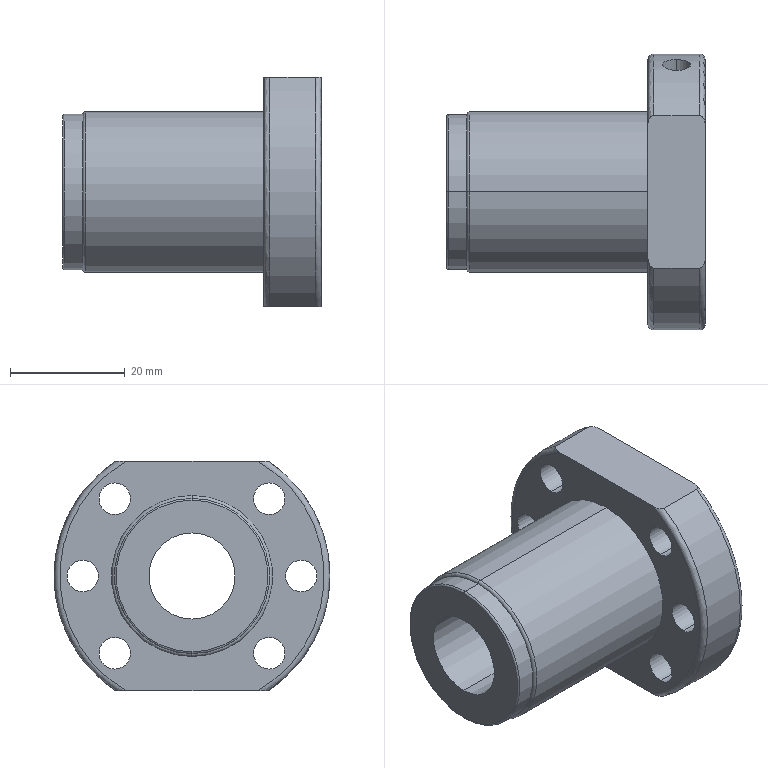Part | SolidWorks | features ICE 3, RefAxis 3, HoleWzd 2, Revolution 2, CirPattern 1 | 1 solid | 108 faces | box 45 x 48 x 40 mm | volume 28053 mm3 | plane 54 | cylinder 40 | torus 8 | cone 6 | commonest cylinder face diameters 5.5 x12 3.3 x10 28 x4 18.2 x3 24.8 x3 4.917 x2